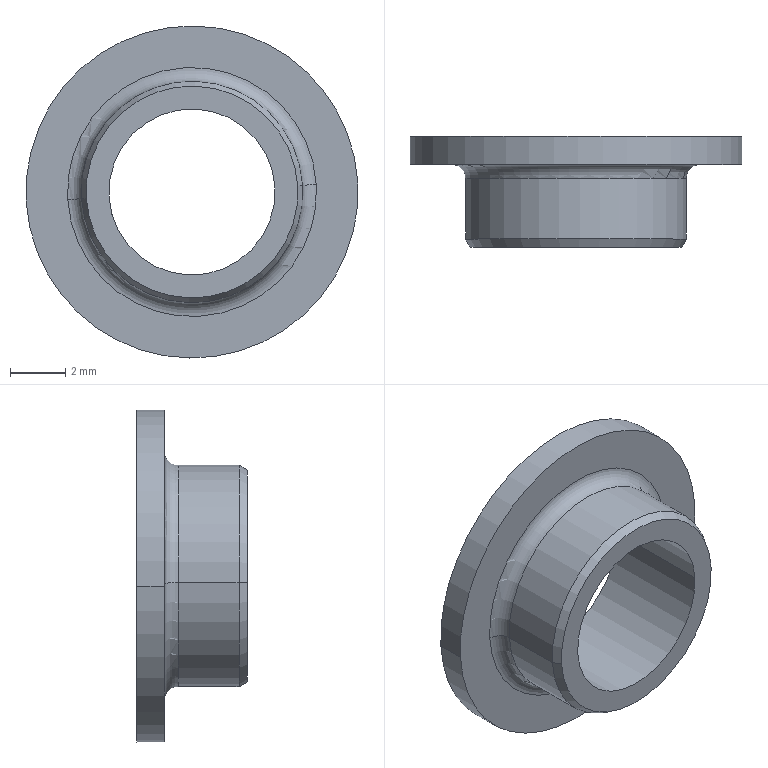Part | NX | features solid 2 | 1 solid | 13 faces | box 12 x 4 x 12 mm | volume 151.539 mm3 | cylinder 6 | plane 3 | cone 2 | torus 2 | commonest cylinder face diameters 6 x2 8 x2 12 x2
STEP:
#1=CARTESIAN_POINT('',(-277.931,63.958,27.464));
#2=VERTEX_POINT('',#1);
#3=CARTESIAN_POINT('',(-289.909,63.958,26.736));
#4=VERTEX_POINT('',#3);
#5=CARTESIAN_POINT('',(-283.92,63.958,27.1));
#6=DIRECTION('',(0.00002097,1.,0.));
#7=DIRECTION('',(0.9982,-0.00002093,0.06061));
#8=AXIS2_PLACEMENT_3D('',#5,#6,#7);
#9=CIRCLE('',#8,6.);
#10=EDGE_CURVE('',#2,#4,#9,.T.);
#11=ORIENTED_EDGE('',*,*,#10,.T.);
#12=CARTESIAN_POINT('',(-283.92,63.958,27.1));
#13=DIRECTION('',(0.00002097,1.,0.));
#14=DIRECTION('',(-0.9982,0.00002093,-0.06061));
#15=AXIS2_PLACEMENT_3D('',#12,#13,#14);
#16=CIRCLE('',#15,6.);
#17=EDGE_CURVE('',#4,#2,#16,.T.);
#18=ORIENTED_EDGE('',*,*,#17,.T.);
#19=EDGE_LOOP('',(#11,#18));
#20=FACE_BOUND('',#19,.T.);
#21=CARTESIAN_POINT('',(-286.915,63.958,26.918));
#22=VERTEX_POINT('',#21);
#23=CARTESIAN_POINT('',(-280.926,63.958,27.282));
#24=VERTEX_POINT('',#23);
#25=CARTESIAN_POINT('',(-283.92,63.958,27.1));
#26=DIRECTION('',(-0.00002097,-1.,0.));
#27=DIRECTION('',(-0.9982,0.00002093,-0.06061));
#28=AXIS2_PLACEMENT_3D('',#25,#26,#27);
#29=CIRCLE('',#28,3.);
#30=EDGE_CURVE('',#22,#24,#29,.T.);
#31=ORIENTED_EDGE('',*,*,#30,.T.);
#32=CARTESIAN_POINT('',(-283.92,63.958,27.1));
#33=DIRECTION('',(-0.00002097,-1.,0.));
#34=DIRECTION('',(0.9982,-0.00002093,0.06061));
#35=AXIS2_PLACEMENT_3D('',#32,#33,#34);
#36=CIRCLE('',#35,3.);
#37=EDGE_CURVE('',#24,#22,#36,.T.);
#38=ORIENTED_EDGE('',*,*,#37,.T.);
#39=EDGE_LOOP('',(#31,#38));
#40=FACE_BOUND('',#39,.T.);
#41=CARTESIAN_POINT('',(-279.429,63.958,27.373));
#42=DIRECTION('',(0.00002097,1.,0.));
#43=DIRECTION('',(0.9982,-0.00002093,0.06061));
#44=AXIS2_PLACEMENT_3D('',#41,#42,#43);
#45=PLANE('',#44);
#46=ADVANCED_FACE('',(#20,#40),#45,.T.);
#47=CARTESIAN_POINT('',(-286.915,59.958,26.918));
#48=VERTEX_POINT('',#47);
#49=CARTESIAN_POINT('',(-280.926,59.958,27.282));
#50=VERTEX_POINT('',#49);
#51=CARTESIAN_POINT('',(-283.92,59.958,27.1));
#52=DIRECTION('',(0.00002097,1.,0.));
#53=DIRECTION('',(-0.9982,0.00002093,-0.06061));
#54=AXIS2_PLACEMENT_3D('',#51,#52,#53);
#55=CIRCLE('',#54,3.);
#56=EDGE_CURVE('',#48,#50,#55,.T.);
#57=ORIENTED_EDGE('',*,*,#56,.F.);
#58=CARTESIAN_POINT('',(-286.915,63.958,26.918));
#59=DIRECTION('',(-0.00002097,-1.,0.));
#60=VECTOR('',#59,1000.);
#61=LINE('',#58,#60);
#62=EDGE_CURVE('',#22,#48,#61,.T.);
#63=ORIENTED_EDGE('',*,*,#62,.F.);
#64=ORIENTED_EDGE('',*,*,#37,.F.);
#65=CARTESIAN_POINT('',(-280.926,59.958,27.282));
#66=DIRECTION('',(0.00002097,1.,0.));
#67=VECTOR('',#66,1000.);
#68=LINE('',#65,#67);
#69=EDGE_CURVE('',#50,#24,#68,.T.);
#70=ORIENTED_EDGE('',*,*,#69,.F.);
#71=EDGE_LOOP('',(#57,#63,#64,#70));
#72=FACE_BOUND('',#71,.T.);
#73=CARTESIAN_POINT('',(-283.92,61.958,27.1));
#74=DIRECTION('',(-0.00002097,-1.,0.));
#75=DIRECTION('',(-0.9982,0.00002093,-0.06061));
#76=AXIS2_PLACEMENT_3D('',#73,#74,#75);
#77=CYLINDRICAL_SURFACE('',#76,3.);
#78=ADVANCED_FACE('',(#72),#77,.F.);
#79=ORIENTED_EDGE('',*,*,#30,.F.);
#80=ORIENTED_EDGE('',*,*,#62,.T.);
#81=CARTESIAN_POINT('',(-283.92,59.958,27.1));
#82=DIRECTION('',(0.00002097,1.,0.));
#83=DIRECTION('',(0.9982,-0.00002093,0.06061));
#84=AXIS2_PLACEMENT_3D('',#81,#82,#83);
#85=CIRCLE('',#84,3.);
#86=EDGE_CURVE('',#50,#48,#85,.T.);
#87=ORIENTED_EDGE('',*,*,#86,.F.);
#88=ORIENTED_EDGE('',*,*,#69,.T.);
#89=EDGE_LOOP('',(#79,#80,#87,#88));
#90=FACE_BOUND('',#89,.T.);
#91=CARTESIAN_POINT('',(-283.92,61.958,27.1));
#92=DIRECTION('',(-0.00002097,-1.,0.));
#93=DIRECTION('',(-0.9982,0.00002093,-0.06061));
#94=AXIS2_PLACEMENT_3D('',#91,#92,#93);
#95=CYLINDRICAL_SURFACE('',#94,3.);
#96=ADVANCED_FACE('',(#90),#95,.F.);
#97=CARTESIAN_POINT('',(-287.74,59.958,26.868));
#98=VERTEX_POINT('',#97);
#99=CARTESIAN_POINT('',(-280.101,59.958,27.332));
#100=VERTEX_POINT('',#99);
#101=CARTESIAN_POINT('',(-283.92,59.958,27.1));
#102=DIRECTION('',(-0.00002097,-1.,0.));
#103=DIRECTION('',(-0.9982,0.00002093,-0.06061));
#104=AXIS2_PLACEMENT_3D('',#101,#102,#103);
#105=CIRCLE('',#104,3.827);
#106=EDGE_CURVE('',#98,#100,#105,.T.);
#107=ORIENTED_EDGE('',*,*,#106,.T.);
#108=CARTESIAN_POINT('',(-283.92,59.958,27.1));
#109=DIRECTION('',(-0.00002097,-1.,0.));
#110=DIRECTION('',(0.9982,-0.00002093,0.06061));
#111=AXIS2_PLACEMENT_3D('',#108,#109,#110);
#112=CIRCLE('',#111,3.827);
#113=EDGE_CURVE('',#100,#98,#112,.T.);
#114=ORIENTED_EDGE('',*,*,#113,.T.);
#115=EDGE_LOOP('',(#107,#114));
#116=FACE_BOUND('',#115,.T.);
#117=ORIENTED_EDGE('',*,*,#86,.T.);
#118=ORIENTED_EDGE('',*,*,#56,.T.);
#119=EDGE_LOOP('',(#117,#118));
#120=FACE_BOUND('',#119,.T.);
#121=CARTESIAN_POINT('',(-280.513,59.958,27.307));
#122=DIRECTION('',(-0.00002097,-1.,0.));
#123=DIRECTION('',(-0.9982,0.00002093,-0.06061));
#124=AXIS2_PLACEMENT_3D('',#121,#122,#123);
#125=PLANE('',#124);
#126=ADVANCED_FACE('',(#116,#120),#125,.T.);
#127=CARTESIAN_POINT('',(-279.928,60.258,27.342));
#128=VERTEX_POINT('',#127);
#129=CARTESIAN_POINT('',(-287.913,60.258,26.858));
#130=VERTEX_POINT('',#129);
#131=CARTESIAN_POINT('',(-283.92,60.258,27.1));
#132=DIRECTION('',(-0.00002097,-1.,0.));
#133=DIRECTION('',(0.9982,-0.00002093,0.06061));
#134=AXIS2_PLACEMENT_3D('',#131,#132,#133);
#135=CIRCLE('',#134,4.);
#136=EDGE_CURVE('',#128,#130,#135,.T.);
#137=ORIENTED_EDGE('',*,*,#136,.T.);
#138=CARTESIAN_POINT('',(-287.913,60.258,26.858));
#139=DIRECTION('',(0.4991,-0.866,0.03031));
#140=VECTOR('',#139,1000.);
#141=LINE('',#138,#140);
#142=EDGE_CURVE('',#130,#98,#141,.T.);
#143=ORIENTED_EDGE('',*,*,#142,.T.);
#144=ORIENTED_EDGE('',*,*,#113,.F.);
#145=CARTESIAN_POINT('',(-280.101,59.958,27.332));
#146=DIRECTION('',(0.4991,0.866,0.03031));
#147=VECTOR('',#146,1000.);
#148=LINE('',#145,#147);
#149=EDGE_CURVE('',#100,#128,#148,.T.);
#150=ORIENTED_EDGE('',*,*,#149,.T.);
#151=EDGE_LOOP('',(#137,#143,#144,#150));
#152=FACE_BOUND('',#151,.T.);
#153=CARTESIAN_POINT('',(-283.92,60.108,27.1));
#154=DIRECTION('',(0.00002097,1.,0.));
#155=DIRECTION('',(-0.9982,0.00002093,-0.06061));
#156=AXIS2_PLACEMENT_3D('',#153,#154,#155);
#157=CONICAL_SURFACE('',#156,3.913,0.5236);
#158=ADVANCED_FACE('',(#152),#157,.T.);
#159=ORIENTED_EDGE('',*,*,#106,.F.);
#160=ORIENTED_EDGE('',*,*,#142,.F.);
#161=CARTESIAN_POINT('',(-283.92,60.258,27.1));
#162=DIRECTION('',(-0.00002097,-1.,0.));
#163=DIRECTION('',(-0.9982,0.00002093,-0.06061));
#164=AXIS2_PLACEMENT_3D('',#161,#162,#163);
#165=CIRCLE('',#164,4.);
#166=EDGE_CURVE('',#130,#128,#165,.T.);
#167=ORIENTED_EDGE('',*,*,#166,.T.);
#168=ORIENTED_EDGE('',*,*,#149,.F.);
#169=EDGE_LOOP('',(#159,#160,#167,#168));
#170=FACE_BOUND('',#169,.T.);
#171=CARTESIAN_POINT('',(-283.92,60.108,27.1));
#172=DIRECTION('',(0.00002097,1.,0.));
#173=DIRECTION('',(-0.9982,0.00002093,-0.06061));
#174=AXIS2_PLACEMENT_3D('',#171,#172,#173);
#175=CONICAL_SURFACE('',#174,3.913,0.5236);
#176=ADVANCED_FACE('',(#170),#175,.T.);
#177=ORIENTED_EDGE('',*,*,#166,.F.);
#178=CARTESIAN_POINT('',(-287.913,62.458,26.858));
#179=VERTEX_POINT('',#178);
#180=CARTESIAN_POINT('',(-287.913,62.458,26.858));
#181=DIRECTION('',(-0.00002097,-1.,0.));
#182=VECTOR('',#181,1000.);
#183=LINE('',#180,#182);
#184=EDGE_CURVE('',#179,#130,#183,.T.);
#185=ORIENTED_EDGE('',*,*,#184,.F.);
#186=CARTESIAN_POINT('',(-279.928,62.458,27.342));
#187=VERTEX_POINT('',#186);
#188=CARTESIAN_POINT('',(-283.92,62.458,27.1));
#189=DIRECTION('',(0.00002097,1.,0.));
#190=DIRECTION('',(0.9982,-0.00002093,0.06061));
#191=AXIS2_PLACEMENT_3D('',#188,#189,#190);
#192=CIRCLE('',#191,4.);
#193=EDGE_CURVE('',#187,#179,#192,.T.);
#194=ORIENTED_EDGE('',*,*,#193,.F.);
#195=CARTESIAN_POINT('',(-279.928,60.258,27.342));
#196=DIRECTION('',(0.00002097,1.,0.));
#197=VECTOR('',#196,1000.);
#198=LINE('',#195,#197);
#199=EDGE_CURVE('',#128,#187,#198,.T.);
#200=ORIENTED_EDGE('',*,*,#199,.F.);
#201=EDGE_LOOP('',(#177,#185,#194,#200));
#202=FACE_BOUND('',#201,.T.);
#203=CARTESIAN_POINT('',(-283.92,61.358,27.1));
#204=DIRECTION('',(-0.00002097,-1.,0.));
#205=DIRECTION('',(-0.9982,0.00002093,-0.06061));
#206=AXIS2_PLACEMENT_3D('',#203,#204,#205);
#207=CYLINDRICAL_SURFACE('',#206,4.);
#208=ADVANCED_FACE('',(#202),#207,.T.);
#209=CARTESIAN_POINT('',(-283.92,62.458,27.1));
#210=DIRECTION('',(0.00002097,1.,0.));
#211=DIRECTION('',(-0.9982,0.00002093,-0.06061));
#212=AXIS2_PLACEMENT_3D('',#209,#210,#211);
#213=CIRCLE('',#212,4.);
#214=EDGE_CURVE('',#179,#187,#213,.T.);
#215=ORIENTED_EDGE('',*,*,#214,.F.);
#216=ORIENTED_EDGE('',*,*,#184,.T.);
#217=ORIENTED_EDGE('',*,*,#136,.F.);
#218=ORIENTED_EDGE('',*,*,#199,.T.);
#219=EDGE_LOOP('',(#215,#216,#217,#218));
#220=FACE_BOUND('',#219,.T.);
#221=CARTESIAN_POINT('',(-283.92,61.358,27.1));
#222=DIRECTION('',(-0.00002097,-1.,0.));
#223=DIRECTION('',(-0.9982,0.00002093,-0.06061));
#224=AXIS2_PLACEMENT_3D('',#221,#222,#223);
#225=CYLINDRICAL_SURFACE('',#224,4.);
#226=ADVANCED_FACE('',(#220),#225,.T.);
#227=ORIENTED_EDGE('',*,*,#214,.T.);
#228=CARTESIAN_POINT('',(-279.429,62.958,27.373));
#229=VERTEX_POINT('',#228);
#230=CARTESIAN_POINT('',(-279.429,62.458,27.373));
#231=DIRECTION('',(-0.06061,0.000001271,0.9982));
#232=DIRECTION('',(0.00002097,1.,0.));
#233=AXIS2_PLACEMENT_3D('',#230,#231,#232);
#234=CIRCLE('',#233,0.5);
#235=EDGE_CURVE('',#229,#187,#234,.T.);
#236=ORIENTED_EDGE('',*,*,#235,.F.);
#237=CARTESIAN_POINT('',(-288.412,62.958,26.827));
#238=VERTEX_POINT('',#237);
#239=CARTESIAN_POINT('',(-283.92,62.958,27.1));
#240=DIRECTION('',(0.00002097,1.,0.));
#241=DIRECTION('',(-0.9982,0.00002093,-0.06061));
#242=AXIS2_PLACEMENT_3D('',#239,#240,#241);
#243=CIRCLE('',#242,4.5);
#244=EDGE_CURVE('',#238,#229,#243,.T.);
#245=ORIENTED_EDGE('',*,*,#244,.F.);
#246=CARTESIAN_POINT('',(-288.412,62.458,26.827));
#247=DIRECTION('',(-0.06061,0.000001271,0.9982));
#248=DIRECTION('',(0.9982,-0.00002093,0.06061));
#249=AXIS2_PLACEMENT_3D('',#246,#247,#248);
#250=CIRCLE('',#249,0.5);
#251=EDGE_CURVE('',#179,#238,#250,.T.);
#252=ORIENTED_EDGE('',*,*,#251,.F.);
#253=EDGE_LOOP('',(#227,#236,#245,#252));
#254=FACE_BOUND('',#253,.T.);
#255=CARTESIAN_POINT('',(-283.92,62.458,27.1));
#256=DIRECTION('',(-0.00002097,-1.,0.));
#257=DIRECTION('',(-0.9982,0.00002093,-0.06061));
#258=AXIS2_PLACEMENT_3D('',#255,#256,#257);
#259=TOROIDAL_SURFACE('',#258,4.5,0.5);
#260=ADVANCED_FACE('',(#254),#259,.F.);
#261=CARTESIAN_POINT('',(-283.92,62.958,27.1));
#262=DIRECTION('',(0.00002097,1.,0.));
#263=DIRECTION('',(0.9982,-0.00002093,0.06061));
#264=AXIS2_PLACEMENT_3D('',#261,#262,#263);
#265=CIRCLE('',#264,4.5);
#266=EDGE_CURVE('',#229,#238,#265,.T.);
#267=ORIENTED_EDGE('',*,*,#266,.F.);
#268=ORIENTED_EDGE('',*,*,#235,.T.);
#269=ORIENTED_EDGE('',*,*,#193,.T.);
#270=ORIENTED_EDGE('',*,*,#251,.T.);
#271=EDGE_LOOP('',(#267,#268,#269,#270));
#272=FACE_BOUND('',#271,.T.);
#273=CARTESIAN_POINT('',(-283.92,62.458,27.1));
#274=DIRECTION('',(-0.00002097,-1.,0.));
#275=DIRECTION('',(-0.9982,0.00002093,-0.06061));
#276=AXIS2_PLACEMENT_3D('',#273,#274,#275);
#277=TOROIDAL_SURFACE('',#276,4.5,0.5);
#278=ADVANCED_FACE('',(#272),#277,.F.);
#279=CARTESIAN_POINT('',(-289.909,62.958,26.736));
#280=VERTEX_POINT('',#279);
#281=CARTESIAN_POINT('',(-277.931,62.958,27.464));
#282=VERTEX_POINT('',#281);
#283=CARTESIAN_POINT('',(-283.92,62.958,27.1));
#284=DIRECTION('',(-0.00002097,-1.,0.));
#285=DIRECTION('',(-0.9982,0.00002093,-0.06061));
#286=AXIS2_PLACEMENT_3D('',#283,#284,#285);
#287=CIRCLE('',#286,6.);
#288=EDGE_CURVE('',#280,#282,#287,.T.);
#289=ORIENTED_EDGE('',*,*,#288,.T.);
#290=CARTESIAN_POINT('',(-283.92,62.958,27.1));
#291=DIRECTION('',(-0.00002097,-1.,0.));
#292=DIRECTION('',(0.9982,-0.00002093,0.06061));
#293=AXIS2_PLACEMENT_3D('',#290,#291,#292);
#294=CIRCLE('',#293,6.);
#295=EDGE_CURVE('',#282,#280,#294,.T.);
#296=ORIENTED_EDGE('',*,*,#295,.T.);
#297=EDGE_LOOP('',(#289,#296));
#298=FACE_BOUND('',#297,.T.);
#299=ORIENTED_EDGE('',*,*,#266,.T.);
#300=ORIENTED_EDGE('',*,*,#244,.T.);
#301=EDGE_LOOP('',(#299,#300));
#302=FACE_BOUND('',#301,.T.);
#303=CARTESIAN_POINT('',(-278.68,62.958,27.418));
#304=DIRECTION('',(-0.00002097,-1.,0.));
#305=DIRECTION('',(-0.9982,0.00002093,-0.06061));
#306=AXIS2_PLACEMENT_3D('',#303,#304,#305);
#307=PLANE('',#306);
#308=ADVANCED_FACE('',(#298,#302),#307,.T.);
#309=ORIENTED_EDGE('',*,*,#17,.F.);
#310=CARTESIAN_POINT('',(-289.909,63.958,26.736));
#311=DIRECTION('',(-0.00002097,-1.,0.));
#312=VECTOR('',#311,1000.);
#313=LINE('',#310,#312);
#314=EDGE_CURVE('',#4,#280,#313,.T.);
#315=ORIENTED_EDGE('',*,*,#314,.T.);
#316=ORIENTED_EDGE('',*,*,#295,.F.);
#317=CARTESIAN_POINT('',(-277.931,62.958,27.464));
#318=DIRECTION('',(0.00002097,1.,0.));
#319=VECTOR('',#318,1000.);
#320=LINE('',#317,#319);
#321=EDGE_CURVE('',#282,#2,#320,.T.);
#322=ORIENTED_EDGE('',*,*,#321,.T.);
#323=EDGE_LOOP('',(#309,#315,#316,#322));
#324=FACE_BOUND('',#323,.T.);
#325=CARTESIAN_POINT('',(-283.92,63.458,27.1));
#326=DIRECTION('',(-0.00002097,-1.,0.));
#327=DIRECTION('',(-0.9982,0.00002093,-0.06061));
#328=AXIS2_PLACEMENT_3D('',#325,#326,#327);
#329=CYLINDRICAL_SURFACE('',#328,6.);
#330=ADVANCED_FACE('',(#324),#329,.T.);
#331=ORIENTED_EDGE('',*,*,#288,.F.);
#332=ORIENTED_EDGE('',*,*,#314,.F.);
#333=ORIENTED_EDGE('',*,*,#10,.F.);
#334=ORIENTED_EDGE('',*,*,#321,.F.);
#335=EDGE_LOOP('',(#331,#332,#333,#334));
#336=FACE_BOUND('',#335,.T.);
#337=CARTESIAN_POINT('',(-283.92,63.458,27.1));
#338=DIRECTION('',(-0.00002097,-1.,0.));
#339=DIRECTION('',(-0.9982,0.00002093,-0.06061));
#340=AXIS2_PLACEMENT_3D('',#337,#338,#339);
#341=CYLINDRICAL_SURFACE('',#340,6.);
#342=ADVANCED_FACE('',(#336),#341,.T.);
#343=CLOSED_SHELL('',(#46,#78,#96,#126,#158,#176,#208,#226,#260,#278,#308,#330,#342));
#344=MANIFOLD_SOLID_BREP('',#343);
#345=(LENGTH_UNIT()NAMED_UNIT(*)SI_UNIT(.MILLI.,.METRE.));
#346=UNCERTAINTY_MEASURE_WITH_UNIT(LENGTH_MEASURE(0.00001),#345,'','');
#347=(NAMED_UNIT(*)PLANE_ANGLE_UNIT()SI_UNIT($,.RADIAN.));
#348=(NAMED_UNIT(*)SI_UNIT($,.STERADIAN.)SOLID_ANGLE_UNIT());
#349=(GEOMETRIC_REPRESENTATION_CONTEXT(3)GLOBAL_UNCERTAINTY_ASSIGNED_CONTEXT((#346))GLOBAL_UNIT_ASSIGNED_CONTEXT((#345,#347,#348))REPRESENTATION_CONTEXT('',''));
#350=ADVANCED_BREP_SHAPE_REPRESENTATION('',(#344),#349);